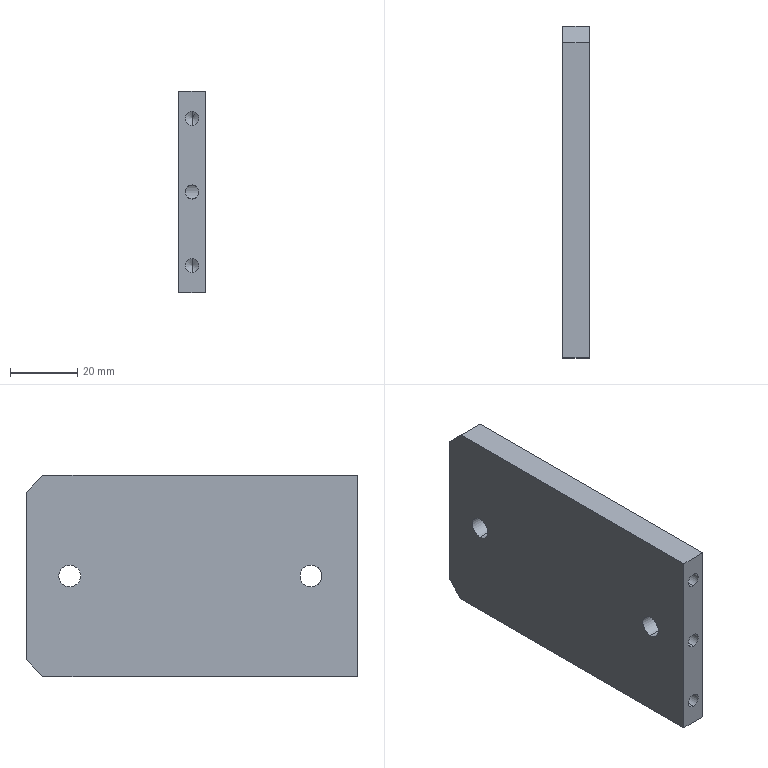Part | STEP file | support plate 25_SUS304 | 1 solid | 22 faces | box 8 x 99 x 60 mm | volume 46238 mm3 | cylinder 10 | plane 8 | cone 4 | commonest cylinder face diameters 4.2 x6 6.5 x4